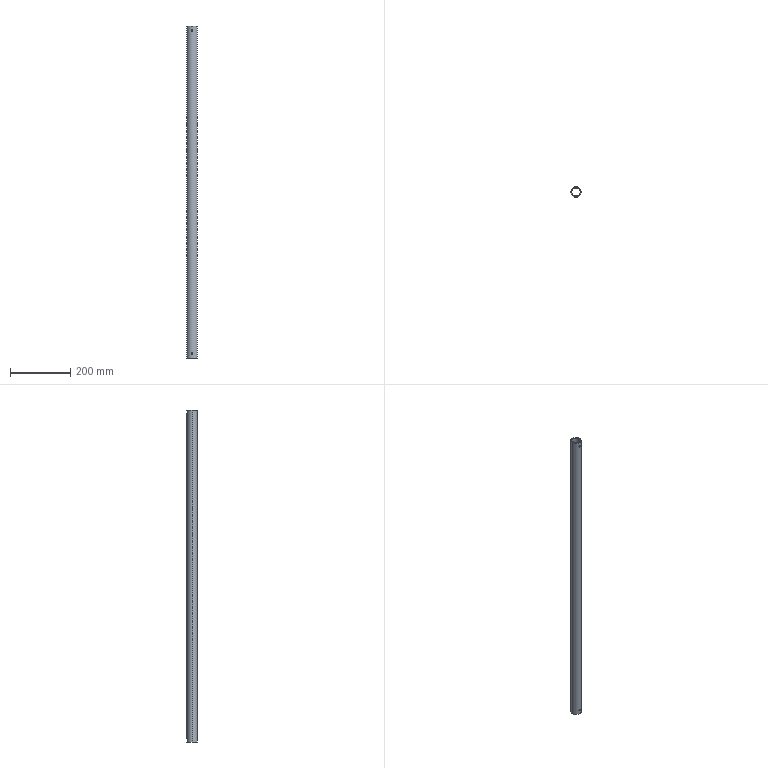Part | SolidWorks | features Extrusion 1, ICE 1 | 1 solid | 14 faces | box 33.7 x 33.7 x 1100 mm | volume 308338 mm3 | cylinder 12 | plane 2 | commonest cylinder face diameters 6 x8 27.9 x2 33.7 x2
STEP:
#1=CARTESIAN_POINT('',(0.,-16.85,12.));
#2=VERTEX_POINT('',#1);
#3=CARTESIAN_POINT('',(0.,-16.85,18.));
#4=VERTEX_POINT('',#3);
#5=CARTESIAN_POINT('',(0.,-16.85,12.));
#6=CARTESIAN_POINT('',(-0.196,-16.85,12.));
#7=CARTESIAN_POINT('',(-0.391,-16.847,12.019));
#8=CARTESIAN_POINT('',(-0.7792,-16.833,12.096));
#9=CARTESIAN_POINT('',(-0.9679,-16.823,12.154));
#10=CARTESIAN_POINT('',(-1.329,-16.798,12.303));
#11=CARTESIAN_POINT('',(-1.504,-16.784,12.397));
#12=CARTESIAN_POINT('',(-1.831,-16.751,12.615));
#13=CARTESIAN_POINT('',(-1.982,-16.734,12.739));
#14=CARTESIAN_POINT('',(-2.258,-16.699,13.016));
#15=CARTESIAN_POINT('',(-2.385,-16.681,13.17));
#16=CARTESIAN_POINT('',(-2.602,-16.648,13.495));
#17=CARTESIAN_POINT('',(-2.695,-16.633,13.667));
#18=CARTESIAN_POINT('',(-2.846,-16.608,14.03));
#19=CARTESIAN_POINT('',(-2.904,-16.598,14.22));
#20=CARTESIAN_POINT('',(-2.98,-16.584,14.604));
#21=CARTESIAN_POINT('',(-3.,-16.581,14.8));
#22=CARTESIAN_POINT('',(-3.,-16.581,15.196));
#23=CARTESIAN_POINT('',(-2.981,-16.584,15.392));
#24=CARTESIAN_POINT('',(-2.905,-16.598,15.776));
#25=CARTESIAN_POINT('',(-2.847,-16.608,15.967));
#26=CARTESIAN_POINT('',(-2.696,-16.633,16.329));
#27=CARTESIAN_POINT('',(-2.604,-16.648,16.502));
#28=CARTESIAN_POINT('',(-2.387,-16.68,16.828));
#29=CARTESIAN_POINT('',(-2.261,-16.698,16.982));
#30=CARTESIAN_POINT('',(-1.847,-16.751,17.396));
#31=CARTESIAN_POINT('',(-1.513,-16.786,17.62));
#32=CARTESIAN_POINT('',(-0.972,-16.823,17.845));
#33=CARTESIAN_POINT('',(-0.7821,-16.833,17.903));
#34=CARTESIAN_POINT('',(-0.3947,-16.846,17.98));
#35=CARTESIAN_POINT('',(-0.1986,-16.85,18.));
#36=CARTESIAN_POINT('',(0.,-16.85,18.));
#37=B_SPLINE_CURVE_WITH_KNOTS('',3,(#5,#6,#7,#8,#9,#10,#11,#12,#13,#14,#15,#16,#17,#18,#19,#20,#21,#22,#23,#24,#25,#26,#27,#28,#29,#30,#31,#32,#33,#34,#35,#36),.UNSPECIFIED.,.F.,.F.,(4,2,2,2,2,2,2,2,2,2,2,2,2,2,2,4),(0.009398,0.009985,0.01057,0.01116,0.01175,0.01233,0.01292,0.01351,0.0141,0.01468,0.01527,0.01586,0.01644,0.01762,0.01821,0.01879),.UNSPECIFIED.);
#38=EDGE_CURVE('',#2,#4,#37,.T.);
#39=ORIENTED_EDGE('',*,*,#38,.F.);
#40=CARTESIAN_POINT('',(0.,-13.95,12.));
#41=VERTEX_POINT('',#40);
#42=CARTESIAN_POINT('',(0.,-16.85,12.));
#43=DIRECTION('',(0.,1.,0.));
#44=VECTOR('',#43,1000.);
#45=LINE('',#42,#44);
#46=EDGE_CURVE('',#2,#41,#45,.T.);
#47=ORIENTED_EDGE('',*,*,#46,.T.);
#48=CARTESIAN_POINT('',(0.,-13.95,18.));
#49=VERTEX_POINT('',#48);
#50=CARTESIAN_POINT('',(0.,-13.95,12.));
#51=CARTESIAN_POINT('',(-0.3921,-13.95,12.));
#52=CARTESIAN_POINT('',(-0.788,-13.932,12.079));
#53=CARTESIAN_POINT('',(-1.33,-13.888,12.304));
#54=CARTESIAN_POINT('',(-1.505,-13.87,12.397));
#55=CARTESIAN_POINT('',(-1.831,-13.83,12.616));
#56=CARTESIAN_POINT('',(-1.982,-13.809,12.739));
#57=CARTESIAN_POINT('',(-2.259,-13.767,13.016));
#58=CARTESIAN_POINT('',(-2.385,-13.745,13.17));
#59=CARTESIAN_POINT('',(-2.602,-13.706,13.494));
#60=CARTESIAN_POINT('',(-2.694,-13.688,13.666));
#61=CARTESIAN_POINT('',(-2.922,-13.642,14.212));
#62=CARTESIAN_POINT('',(-3.,-13.624,14.603));
#63=CARTESIAN_POINT('',(-3.,-13.624,15.197));
#64=CARTESIAN_POINT('',(-2.981,-13.628,15.392));
#65=CARTESIAN_POINT('',(-2.904,-13.644,15.776));
#66=CARTESIAN_POINT('',(-2.846,-13.657,15.968));
#67=CARTESIAN_POINT('',(-2.696,-13.687,16.33));
#68=CARTESIAN_POINT('',(-2.604,-13.705,16.502));
#69=CARTESIAN_POINT('',(-2.386,-13.745,16.829));
#70=CARTESIAN_POINT('',(-2.26,-13.766,16.982));
#71=CARTESIAN_POINT('',(-1.847,-13.83,17.396));
#72=CARTESIAN_POINT('',(-1.514,-13.872,17.619));
#73=CARTESIAN_POINT('',(-0.9725,-13.917,17.845));
#74=CARTESIAN_POINT('',(-0.7819,-13.929,17.903));
#75=CARTESIAN_POINT('',(-0.3949,-13.946,17.98));
#76=CARTESIAN_POINT('',(-0.1988,-13.95,18.));
#77=CARTESIAN_POINT('',(0.,-13.95,18.));
#78=B_SPLINE_CURVE_WITH_KNOTS('',3,(#50,#51,#52,#53,#54,#55,#56,#57,#58,#59,#60,#61,#62,#63,#64,#65,#66,#67,#68,#69,#70,#71,#72,#73,#74,#75,#76,#77),.UNSPECIFIED.,.F.,.F.,(4,2,2,2,2,2,2,2,2,2,2,2,2,4),(0.009407,0.01058,0.01117,0.01176,0.01235,0.01293,0.01411,0.0147,0.01528,0.01587,0.01646,0.01764,0.01822,0.01881),.UNSPECIFIED.);
#79=EDGE_CURVE('',#41,#49,#78,.T.);
#80=ORIENTED_EDGE('',*,*,#79,.T.);
#81=CARTESIAN_POINT('',(0.,-16.85,18.));
#82=DIRECTION('',(0.,1.,0.));
#83=VECTOR('',#82,1000.);
#84=LINE('',#81,#83);
#85=EDGE_CURVE('',#4,#49,#84,.T.);
#86=ORIENTED_EDGE('',*,*,#85,.F.);
#87=EDGE_LOOP('',(#39,#47,#80,#86));
#88=FACE_OUTER_BOUND('',#87,.T.);
#89=CARTESIAN_POINT('',(0.,-16.85,15.));
#90=DIRECTION('',(0.,1.,0.));
#91=DIRECTION('',(0.,0.,1.));
#92=AXIS2_PLACEMENT_3D('',#89,#90,#91);
#93=CYLINDRICAL_SURFACE('',#92,3.);
#94=ADVANCED_FACE('',(#88),#93,.F.);
#95=CARTESIAN_POINT('',(0.,13.95,18.));
#96=VERTEX_POINT('',#95);
#97=CARTESIAN_POINT('',(0.,13.95,12.));
#98=VERTEX_POINT('',#97);
#99=CARTESIAN_POINT('',(0.,13.95,18.));
#100=CARTESIAN_POINT('',(-0.1988,13.95,18.));
#101=CARTESIAN_POINT('',(-0.3942,13.946,17.98));
#102=CARTESIAN_POINT('',(-0.7785,13.93,17.904));
#103=CARTESIAN_POINT('',(-0.9694,13.917,17.846));
#104=CARTESIAN_POINT('',(-1.332,13.887,17.695));
#105=CARTESIAN_POINT('',(-1.505,13.87,17.603));
#106=CARTESIAN_POINT('',(-1.83,13.83,17.385));
#107=CARTESIAN_POINT('',(-1.984,13.809,17.259));
#108=CARTESIAN_POINT('',(-2.26,13.766,16.983));
#109=CARTESIAN_POINT('',(-2.384,13.745,16.832));
#110=CARTESIAN_POINT('',(-2.603,13.705,16.504));
#111=CARTESIAN_POINT('',(-2.696,13.687,16.331));
#112=CARTESIAN_POINT('',(-2.846,13.657,15.97));
#113=CARTESIAN_POINT('',(-2.904,13.645,15.78));
#114=CARTESIAN_POINT('',(-2.981,13.628,15.393));
#115=CARTESIAN_POINT('',(-3.,13.624,15.198));
#116=CARTESIAN_POINT('',(-3.,13.624,14.805));
#117=CARTESIAN_POINT('',(-2.98,13.628,14.605));
#118=CARTESIAN_POINT('',(-2.904,13.645,14.22));
#119=CARTESIAN_POINT('',(-2.847,13.657,14.033));
#120=CARTESIAN_POINT('',(-2.696,13.687,13.669));
#121=CARTESIAN_POINT('',(-2.602,13.706,13.494));
#122=CARTESIAN_POINT('',(-2.385,13.745,13.17));
#123=CARTESIAN_POINT('',(-2.26,13.766,13.018));
#124=CARTESIAN_POINT('',(-1.982,13.809,12.739));
#125=CARTESIAN_POINT('',(-1.831,13.83,12.615));
#126=CARTESIAN_POINT('',(-1.506,13.869,12.398));
#127=CARTESIAN_POINT('',(-1.331,13.888,12.304));
#128=CARTESIAN_POINT('',(-0.9682,13.918,12.154));
#129=CARTESIAN_POINT('',(-0.7811,13.929,12.097));
#130=CARTESIAN_POINT('',(-0.3953,13.946,12.02));
#131=CARTESIAN_POINT('',(-0.1961,13.95,12.));
#132=CARTESIAN_POINT('',(0.,13.95,12.));
#133=B_SPLINE_CURVE_WITH_KNOTS('',3,(#99,#100,#101,#102,#103,#104,#105,#106,#107,#108,#109,#110,#111,#112,#113,#114,#115,#116,#117,#118,#119,#120,#121,#122,#123,#124,#125,#126,#127,#128,#129,#130,#131,#132),.UNSPECIFIED.,.F.,.F.,(4,2,2,2,2,2,2,2,2,2,2,2,2,2,2,2,4),(0.,0.0005879,0.001176,0.001764,0.002352,0.00294,0.003528,0.004116,0.004703,0.005291,0.005879,0.006467,0.007055,0.007643,0.008231,0.008819,0.009407),.UNSPECIFIED.);
#134=EDGE_CURVE('',#96,#98,#133,.T.);
#135=ORIENTED_EDGE('',*,*,#134,.T.);
#136=CARTESIAN_POINT('',(0.,16.85,12.));
#137=VERTEX_POINT('',#136);
#138=CARTESIAN_POINT('',(0.,-16.85,12.));
#139=DIRECTION('',(0.,1.,0.));
#140=VECTOR('',#139,1000.);
#141=LINE('',#138,#140);
#142=EDGE_CURVE('',#98,#137,#141,.T.);
#143=ORIENTED_EDGE('',*,*,#142,.T.);
#144=CARTESIAN_POINT('',(0.,16.85,18.));
#145=VERTEX_POINT('',#144);
#146=CARTESIAN_POINT('',(0.,16.85,18.));
#147=CARTESIAN_POINT('',(-0.1986,16.85,18.));
#148=CARTESIAN_POINT('',(-0.3939,16.846,17.98));
#149=CARTESIAN_POINT('',(-0.7779,16.833,17.904));
#150=CARTESIAN_POINT('',(-0.9687,16.823,17.846));
#151=CARTESIAN_POINT('',(-1.332,16.798,17.695));
#152=CARTESIAN_POINT('',(-1.504,16.784,17.603));
#153=CARTESIAN_POINT('',(-1.83,16.751,17.385));
#154=CARTESIAN_POINT('',(-1.984,16.733,17.259));
#155=CARTESIAN_POINT('',(-2.26,16.698,16.983));
#156=CARTESIAN_POINT('',(-2.384,16.681,16.832));
#157=CARTESIAN_POINT('',(-2.603,16.648,16.504));
#158=CARTESIAN_POINT('',(-2.696,16.633,16.33));
#159=CARTESIAN_POINT('',(-2.846,16.608,15.969));
#160=CARTESIAN_POINT('',(-2.904,16.598,15.78));
#161=CARTESIAN_POINT('',(-2.981,16.584,15.392));
#162=CARTESIAN_POINT('',(-3.,16.581,15.197));
#163=CARTESIAN_POINT('',(-3.,16.581,14.805));
#164=CARTESIAN_POINT('',(-2.98,16.584,14.606));
#165=CARTESIAN_POINT('',(-2.904,16.598,14.221));
#166=CARTESIAN_POINT('',(-2.847,16.608,14.034));
#167=CARTESIAN_POINT('',(-2.696,16.633,13.67));
#168=CARTESIAN_POINT('',(-2.602,16.648,13.495));
#169=CARTESIAN_POINT('',(-2.385,16.681,13.17));
#170=CARTESIAN_POINT('',(-2.261,16.698,13.018));
#171=CARTESIAN_POINT('',(-1.982,16.734,12.739));
#172=CARTESIAN_POINT('',(-1.831,16.751,12.615));
#173=CARTESIAN_POINT('',(-1.506,16.783,12.398));
#174=CARTESIAN_POINT('',(-1.33,16.798,12.304));
#175=CARTESIAN_POINT('',(-0.9675,16.823,12.154));
#176=CARTESIAN_POINT('',(-0.7805,16.833,12.097));
#177=CARTESIAN_POINT('',(-0.3951,16.846,12.02));
#178=CARTESIAN_POINT('',(-0.196,16.85,12.));
#179=CARTESIAN_POINT('',(0.,16.85,12.));
#180=B_SPLINE_CURVE_WITH_KNOTS('',3,(#146,#147,#148,#149,#150,#151,#152,#153,#154,#155,#156,#157,#158,#159,#160,#161,#162,#163,#164,#165,#166,#167,#168,#169,#170,#171,#172,#173,#174,#175,#176,#177,#178,#179),.UNSPECIFIED.,.F.,.F.,(4,2,2,2,2,2,2,2,2,2,2,2,2,2,2,2,4),(0.,0.0005874,0.001175,0.001762,0.00235,0.002937,0.003524,0.004112,0.004699,0.005286,0.005874,0.006461,0.007049,0.007636,0.008223,0.008811,0.009398),.UNSPECIFIED.);
#181=EDGE_CURVE('',#145,#137,#180,.T.);
#182=ORIENTED_EDGE('',*,*,#181,.F.);
#183=CARTESIAN_POINT('',(0.,-16.85,18.));
#184=DIRECTION('',(0.,1.,0.));
#185=VECTOR('',#184,1000.);
#186=LINE('',#183,#185);
#187=EDGE_CURVE('',#96,#145,#186,.T.);
#188=ORIENTED_EDGE('',*,*,#187,.F.);
#189=EDGE_LOOP('',(#135,#143,#182,#188));
#190=FACE_OUTER_BOUND('',#189,.T.);
#191=CARTESIAN_POINT('',(0.,-16.85,15.));
#192=DIRECTION('',(0.,1.,0.));
#193=DIRECTION('',(0.,0.,1.));
#194=AXIS2_PLACEMENT_3D('',#191,#192,#193);
#195=CYLINDRICAL_SURFACE('',#194,3.);
#196=ADVANCED_FACE('',(#190),#195,.F.);
#197=CARTESIAN_POINT('',(0.,-16.85,1082.));
#198=VERTEX_POINT('',#197);
#199=CARTESIAN_POINT('',(0.,-16.85,1088.));
#200=VERTEX_POINT('',#199);
#201=CARTESIAN_POINT('',(0.,-16.85,1082.));
#202=CARTESIAN_POINT('',(-0.196,-16.85,1082.));
#203=CARTESIAN_POINT('',(-0.391,-16.847,1082.019));
#204=CARTESIAN_POINT('',(-0.7792,-16.833,1082.096));
#205=CARTESIAN_POINT('',(-0.9679,-16.823,1082.154));
#206=CARTESIAN_POINT('',(-1.329,-16.798,1082.303));
#207=CARTESIAN_POINT('',(-1.504,-16.784,1082.397));
#208=CARTESIAN_POINT('',(-1.831,-16.751,1082.615));
#209=CARTESIAN_POINT('',(-1.982,-16.734,1082.739));
#210=CARTESIAN_POINT('',(-2.258,-16.699,1083.016));
#211=CARTESIAN_POINT('',(-2.385,-16.681,1083.17));
#212=CARTESIAN_POINT('',(-2.602,-16.648,1083.495));
#213=CARTESIAN_POINT('',(-2.695,-16.633,1083.667));
#214=CARTESIAN_POINT('',(-2.846,-16.608,1084.03));
#215=CARTESIAN_POINT('',(-2.904,-16.598,1084.22));
#216=CARTESIAN_POINT('',(-2.98,-16.584,1084.604));
#217=CARTESIAN_POINT('',(-3.,-16.581,1084.8));
#218=CARTESIAN_POINT('',(-3.,-16.581,1085.196));
#219=CARTESIAN_POINT('',(-2.981,-16.584,1085.392));
#220=CARTESIAN_POINT('',(-2.905,-16.598,1085.776));
#221=CARTESIAN_POINT('',(-2.847,-16.608,1085.967));
#222=CARTESIAN_POINT('',(-2.696,-16.633,1086.329));
#223=CARTESIAN_POINT('',(-2.604,-16.648,1086.502));
#224=CARTESIAN_POINT('',(-2.387,-16.68,1086.828));
#225=CARTESIAN_POINT('',(-2.261,-16.698,1086.982));
#226=CARTESIAN_POINT('',(-1.847,-16.751,1087.396));
#227=CARTESIAN_POINT('',(-1.513,-16.786,1087.62));
#228=CARTESIAN_POINT('',(-0.972,-16.823,1087.845));
#229=CARTESIAN_POINT('',(-0.7821,-16.833,1087.903));
#230=CARTESIAN_POINT('',(-0.3947,-16.846,1087.98));
#231=CARTESIAN_POINT('',(-0.1986,-16.85,1088.));
#232=CARTESIAN_POINT('',(0.,-16.85,1088.));
#233=B_SPLINE_CURVE_WITH_KNOTS('',3,(#201,#202,#203,#204,#205,#206,#207,#208,#209,#210,#211,#212,#213,#214,#215,#216,#217,#218,#219,#220,#221,#222,#223,#224,#225,#226,#227,#228,#229,#230,#231,#232),.UNSPECIFIED.,.F.,.F.,(4,2,2,2,2,2,2,2,2,2,2,2,2,2,2,4),(0.009398,0.009985,0.01057,0.01116,0.01175,0.01233,0.01292,0.01351,0.0141,0.01468,0.01527,0.01586,0.01644,0.01762,0.01821,0.01879),.UNSPECIFIED.);
#234=EDGE_CURVE('',#198,#200,#233,.T.);
#235=ORIENTED_EDGE('',*,*,#234,.F.);
#236=CARTESIAN_POINT('',(0.,-13.95,1082.));
#237=VERTEX_POINT('',#236);
#238=CARTESIAN_POINT('',(0.,-16.85,1082.));
#239=DIRECTION('',(0.,1.,0.));
#240=VECTOR('',#239,1000.);
#241=LINE('',#238,#240);
#242=EDGE_CURVE('',#198,#237,#241,.T.);
#243=ORIENTED_EDGE('',*,*,#242,.T.);
#244=CARTESIAN_POINT('',(0.,-13.95,1088.));
#245=VERTEX_POINT('',#244);
#246=CARTESIAN_POINT('',(0.,-13.95,1082.));
#247=CARTESIAN_POINT('',(-0.3921,-13.95,1082.));
#248=CARTESIAN_POINT('',(-0.788,-13.932,1082.079));
#249=CARTESIAN_POINT('',(-1.33,-13.888,1082.304));
#250=CARTESIAN_POINT('',(-1.505,-13.87,1082.397));
#251=CARTESIAN_POINT('',(-1.831,-13.83,1082.616));
#252=CARTESIAN_POINT('',(-1.982,-13.809,1082.739));
#253=CARTESIAN_POINT('',(-2.259,-13.767,1083.016));
#254=CARTESIAN_POINT('',(-2.385,-13.745,1083.17));
#255=CARTESIAN_POINT('',(-2.602,-13.706,1083.494));
#256=CARTESIAN_POINT('',(-2.694,-13.688,1083.666));
#257=CARTESIAN_POINT('',(-2.922,-13.642,1084.212));
#258=CARTESIAN_POINT('',(-3.,-13.624,1084.603));
#259=CARTESIAN_POINT('',(-3.,-13.624,1085.197));
#260=CARTESIAN_POINT('',(-2.981,-13.628,1085.392));
#261=CARTESIAN_POINT('',(-2.904,-13.644,1085.776));
#262=CARTESIAN_POINT('',(-2.846,-13.657,1085.968));
#263=CARTESIAN_POINT('',(-2.696,-13.687,1086.33));
#264=CARTESIAN_POINT('',(-2.604,-13.705,1086.502));
#265=CARTESIAN_POINT('',(-2.386,-13.745,1086.829));
#266=CARTESIAN_POINT('',(-2.26,-13.766,1086.982));
#267=CARTESIAN_POINT('',(-1.847,-13.83,1087.396));
#268=CARTESIAN_POINT('',(-1.514,-13.872,1087.619));
#269=CARTESIAN_POINT('',(-0.9725,-13.917,1087.845));
#270=CARTESIAN_POINT('',(-0.7819,-13.929,1087.903));
#271=CARTESIAN_POINT('',(-0.3949,-13.946,1087.98));
#272=CARTESIAN_POINT('',(-0.1988,-13.95,1088.));
#273=CARTESIAN_POINT('',(0.,-13.95,1088.));
#274=B_SPLINE_CURVE_WITH_KNOTS('',3,(#246,#247,#248,#249,#250,#251,#252,#253,#254,#255,#256,#257,#258,#259,#260,#261,#262,#263,#264,#265,#266,#267,#268,#269,#270,#271,#272,#273),.UNSPECIFIED.,.F.,.F.,(4,2,2,2,2,2,2,2,2,2,2,2,2,4),(0.009407,0.01058,0.01117,0.01176,0.01235,0.01293,0.01411,0.0147,0.01528,0.01587,0.01646,0.01764,0.01822,0.01881),.UNSPECIFIED.);
#275=EDGE_CURVE('',#237,#245,#274,.T.);
#276=ORIENTED_EDGE('',*,*,#275,.T.);
#277=CARTESIAN_POINT('',(0.,-16.85,1088.));
#278=DIRECTION('',(0.,1.,0.));
#279=VECTOR('',#278,1000.);
#280=LINE('',#277,#279);
#281=EDGE_CURVE('',#200,#245,#280,.T.);
#282=ORIENTED_EDGE('',*,*,#281,.F.);
#283=EDGE_LOOP('',(#235,#243,#276,#282));
#284=FACE_OUTER_BOUND('',#283,.T.);
#285=CARTESIAN_POINT('',(0.,-16.85,1085.));
#286=DIRECTION('',(0.,1.,0.));
#287=DIRECTION('',(0.,0.,1.));
#288=AXIS2_PLACEMENT_3D('',#285,#286,#287);
#289=CYLINDRICAL_SURFACE('',#288,3.);
#290=ADVANCED_FACE('',(#284),#289,.F.);
#291=CARTESIAN_POINT('',(0.,13.95,1088.));
#292=VERTEX_POINT('',#291);
#293=CARTESIAN_POINT('',(0.,13.95,1082.));
#294=VERTEX_POINT('',#293);
#295=CARTESIAN_POINT('',(0.,13.95,1088.));
#296=CARTESIAN_POINT('',(-0.1988,13.95,1088.));
#297=CARTESIAN_POINT('',(-0.3942,13.946,1087.98));
#298=CARTESIAN_POINT('',(-0.7785,13.93,1087.904));
#299=CARTESIAN_POINT('',(-0.9694,13.917,1087.846));
#300=CARTESIAN_POINT('',(-1.332,13.887,1087.695));
#301=CARTESIAN_POINT('',(-1.505,13.87,1087.603));
#302=CARTESIAN_POINT('',(-1.83,13.83,1087.385));
#303=CARTESIAN_POINT('',(-1.984,13.809,1087.259));
#304=CARTESIAN_POINT('',(-2.26,13.766,1086.983));
#305=CARTESIAN_POINT('',(-2.384,13.745,1086.832));
#306=CARTESIAN_POINT('',(-2.603,13.705,1086.504));
#307=CARTESIAN_POINT('',(-2.696,13.687,1086.331));
#308=CARTESIAN_POINT('',(-2.846,13.657,1085.97));
#309=CARTESIAN_POINT('',(-2.904,13.645,1085.78));
#310=CARTESIAN_POINT('',(-2.981,13.628,1085.393));
#311=CARTESIAN_POINT('',(-3.,13.624,1085.198));
#312=CARTESIAN_POINT('',(-3.,13.624,1084.805));
#313=CARTESIAN_POINT('',(-2.98,13.628,1084.605));
#314=CARTESIAN_POINT('',(-2.904,13.645,1084.22));
#315=CARTESIAN_POINT('',(-2.847,13.657,1084.033));
#316=CARTESIAN_POINT('',(-2.696,13.687,1083.669));
#317=CARTESIAN_POINT('',(-2.602,13.706,1083.494));
#318=CARTESIAN_POINT('',(-2.385,13.745,1083.17));
#319=CARTESIAN_POINT('',(-2.26,13.766,1083.018));
#320=CARTESIAN_POINT('',(-1.982,13.809,1082.739));
#321=CARTESIAN_POINT('',(-1.831,13.83,1082.615));
#322=CARTESIAN_POINT('',(-1.506,13.869,1082.398));
#323=CARTESIAN_POINT('',(-1.331,13.888,1082.304));
#324=CARTESIAN_POINT('',(-0.9682,13.918,1082.154));
#325=CARTESIAN_POINT('',(-0.7811,13.929,1082.097));
#326=CARTESIAN_POINT('',(-0.3953,13.946,1082.02));
#327=CARTESIAN_POINT('',(-0.1961,13.95,1082.));
#328=CARTESIAN_POINT('',(0.,13.95,1082.));
#329=B_SPLINE_CURVE_WITH_KNOTS('',3,(#295,#296,#297,#298,#299,#300,#301,#302,#303,#304,#305,#306,#307,#308,#309,#310,#311,#312,#313,#314,#315,#316,#317,#318,#319,#320,#321,#322,#323,#324,#325,#326,#327,#328),.UNSPECIFIED.,.F.,.F.,(4,2,2,2,2,2,2,2,2,2,2,2,2,2,2,2,4),(0.,0.0005879,0.001176,0.001764,0.002352,0.00294,0.003528,0.004116,0.004703,0.005291,0.005879,0.006467,0.007055,0.007643,0.008231,0.008819,0.009407),.UNSPECIFIED.);
#330=EDGE_CURVE('',#292,#294,#329,.T.);
#331=ORIENTED_EDGE('',*,*,#330,.T.);
#332=CARTESIAN_POINT('',(0.,16.85,1082.));
#333=VERTEX_POINT('',#332);
#334=CARTESIAN_POINT('',(0.,-16.85,1082.));
#335=DIRECTION('',(0.,1.,0.));
#336=VECTOR('',#335,1000.);
#337=LINE('',#334,#336);
#338=EDGE_CURVE('',#294,#333,#337,.T.);
#339=ORIENTED_EDGE('',*,*,#338,.T.);
#340=CARTESIAN_POINT('',(0.,16.85,1088.));
#341=VERTEX_POINT('',#340);
#342=CARTESIAN_POINT('',(0.,16.85,1088.));
#343=CARTESIAN_POINT('',(-0.1986,16.85,1088.));
#344=CARTESIAN_POINT('',(-0.3939,16.846,1087.98));
#345=CARTESIAN_POINT('',(-0.7779,16.833,1087.904));
#346=CARTESIAN_POINT('',(-0.9687,16.823,1087.846));
#347=CARTESIAN_POINT('',(-1.332,16.798,1087.695));
#348=CARTESIAN_POINT('',(-1.504,16.784,1087.603));
#349=CARTESIAN_POINT('',(-1.83,16.751,1087.385));
#350=CARTESIAN_POINT('',(-1.984,16.733,1087.259));
#351=CARTESIAN_POINT('',(-2.26,16.698,1086.983));
#352=CARTESIAN_POINT('',(-2.384,16.681,1086.832));
#353=CARTESIAN_POINT('',(-2.603,16.648,1086.504));
#354=CARTESIAN_POINT('',(-2.696,16.633,1086.33));
#355=CARTESIAN_POINT('',(-2.846,16.608,1085.969));
#356=CARTESIAN_POINT('',(-2.904,16.598,1085.78));
#357=CARTESIAN_POINT('',(-2.981,16.584,1085.392));
#358=CARTESIAN_POINT('',(-3.,16.581,1085.197));
#359=CARTESIAN_POINT('',(-3.,16.581,1084.805));
#360=CARTESIAN_POINT('',(-2.98,16.584,1084.606));
#361=CARTESIAN_POINT('',(-2.904,16.598,1084.221));
#362=CARTESIAN_POINT('',(-2.847,16.608,1084.034));
#363=CARTESIAN_POINT('',(-2.696,16.633,1083.67));
#364=CARTESIAN_POINT('',(-2.602,16.648,1083.495));
#365=CARTESIAN_POINT('',(-2.385,16.681,1083.17));
#366=CARTESIAN_POINT('',(-2.261,16.698,1083.018));
#367=CARTESIAN_POINT('',(-1.982,16.734,1082.739));
#368=CARTESIAN_POINT('',(-1.831,16.751,1082.615));
#369=CARTESIAN_POINT('',(-1.506,16.783,1082.398));
#370=CARTESIAN_POINT('',(-1.33,16.798,1082.304));
#371=CARTESIAN_POINT('',(-0.9675,16.823,1082.154));
#372=CARTESIAN_POINT('',(-0.7805,16.833,1082.097));
#373=CARTESIAN_POINT('',(-0.3951,16.846,1082.02));
#374=CARTESIAN_POINT('',(-0.196,16.85,1082.));
#375=CARTESIAN_POINT('',(0.,16.85,1082.));
#376=B_SPLINE_CURVE_WITH_KNOTS('',3,(#342,#343,#344,#345,#346,#347,#348,#349,#350,#351,#352,#353,#354,#355,#356,#357,#358,#359,#360,#361,#362,#363,#364,#365,#366,#367,#368,#369,#370,#371,#372,#373,#374,#375),.UNSPECIFIED.,.F.,.F.,(4,2,2,2,2,2,2,2,2,2,2,2,2,2,2,2,4),(0.,0.0005874,0.001175,0.001762,0.00235,0.002937,0.003524,0.004112,0.004699,0.005286,0.005874,0.006461,0.007049,0.007636,0.008223,0.008811,0.009398),.UNSPECIFIED.);
#377=EDGE_CURVE('',#341,#333,#376,.T.);
#378=ORIENTED_EDGE('',*,*,#377,.F.);
#379=CARTESIAN_POINT('',(0.,-16.85,1088.));
#380=DIRECTION('',(0.,1.,0.));
#381=VECTOR('',#380,1000.);
#382=LINE('',#379,#381);
#383=EDGE_CURVE('',#292,#341,#382,.T.);
#384=ORIENTED_EDGE('',*,*,#383,.F.);
#385=EDGE_LOOP('',(#331,#339,#378,#384));
#386=FACE_OUTER_BOUND('',#385,.T.);
#387=CARTESIAN_POINT('',(0.,-16.85,1085.));
#388=DIRECTION('',(0.,1.,0.));
#389=DIRECTION('',(0.,0.,1.));
#390=AXIS2_PLACEMENT_3D('',#387,#388,#389);
#391=CYLINDRICAL_SURFACE('',#390,3.);
#392=ADVANCED_FACE('',(#386),#391,.F.);
#393=CARTESIAN_POINT('',(0.,-13.95,1088.));
#394=CARTESIAN_POINT('',(0.1988,-13.95,1088.));
#395=CARTESIAN_POINT('',(0.3942,-13.946,1087.98));
#396=CARTESIAN_POINT('',(0.7785,-13.93,1087.904));
#397=CARTESIAN_POINT('',(0.9694,-13.917,1087.846));
#398=CARTESIAN_POINT('',(1.332,-13.887,1087.695));
#399=CARTESIAN_POINT('',(1.505,-13.87,1087.603));
#400=CARTESIAN_POINT('',(1.83,-13.83,1087.385));
#401=CARTESIAN_POINT('',(1.984,-13.809,1087.259));
#402=CARTESIAN_POINT('',(2.26,-13.766,1086.983));
#403=CARTESIAN_POINT('',(2.384,-13.745,1086.832));
#404=CARTESIAN_POINT('',(2.603,-13.705,1086.504));
#405=CARTESIAN_POINT('',(2.696,-13.687,1086.331));
#406=CARTESIAN_POINT('',(2.846,-13.657,1085.97));
#407=CARTESIAN_POINT('',(2.904,-13.645,1085.78));
#408=CARTESIAN_POINT('',(2.981,-13.628,1085.393));
#409=CARTESIAN_POINT('',(3.,-13.624,1085.198));
#410=CARTESIAN_POINT('',(3.,-13.624,1084.805));
#411=CARTESIAN_POINT('',(2.98,-13.628,1084.605));
#412=CARTESIAN_POINT('',(2.904,-13.645,1084.22));
#413=CARTESIAN_POINT('',(2.847,-13.657,1084.033));
#414=CARTESIAN_POINT('',(2.696,-13.687,1083.669));
#415=CARTESIAN_POINT('',(2.602,-13.706,1083.494));
#416=CARTESIAN_POINT('',(2.385,-13.745,1083.17));
#417=CARTESIAN_POINT('',(2.26,-13.766,1083.018));
#418=CARTESIAN_POINT('',(1.982,-13.809,1082.739));
#419=CARTESIAN_POINT('',(1.831,-13.83,1082.615));
#420=CARTESIAN_POINT('',(1.506,-13.869,1082.398));
#421=CARTESIAN_POINT('',(1.331,-13.888,1082.304));
#422=CARTESIAN_POINT('',(0.9682,-13.918,1082.154));
#423=CARTESIAN_POINT('',(0.7811,-13.929,1082.097));
#424=CARTESIAN_POINT('',(0.3953,-13.946,1082.02));
#425=CARTESIAN_POINT('',(0.1961,-13.95,1082.));
#426=CARTESIAN_POINT('',(0.,-13.95,1082.));
#427=B_SPLINE_CURVE_WITH_KNOTS('',3,(#393,#394,#395,#396,#397,#398,#399,#400,#401,#402,#403,#404,#405,#406,#407,#408,#409,#410,#411,#412,#413,#414,#415,#416,#417,#418,#419,#420,#421,#422,#423,#424,#425,#426),.UNSPECIFIED.,.F.,.F.,(4,2,2,2,2,2,2,2,2,2,2,2,2,2,2,2,4),(0.,0.0005879,0.001176,0.001764,0.002352,0.00294,0.003528,0.004116,0.004703,0.005291,0.005879,0.006467,0.007055,0.007643,0.008231,0.008819,0.009407),.UNSPECIFIED.);
#428=EDGE_CURVE('',#245,#237,#427,.T.);
#429=ORIENTED_EDGE('',*,*,#428,.F.);
#430=ORIENTED_EDGE('',*,*,#275,.F.);
#431=EDGE_LOOP('',(#429,#430));
#432=FACE_BOUND('',#431,.T.);
#433=CARTESIAN_POINT('',(0.,-13.95,18.));
#434=CARTESIAN_POINT('',(0.1988,-13.95,18.));
#435=CARTESIAN_POINT('',(0.3942,-13.946,17.98));
#436=CARTESIAN_POINT('',(0.7785,-13.93,17.904));
#437=CARTESIAN_POINT('',(0.9694,-13.917,17.846));
#438=CARTESIAN_POINT('',(1.332,-13.887,17.695));
#439=CARTESIAN_POINT('',(1.505,-13.87,17.603));
#440=CARTESIAN_POINT('',(1.83,-13.83,17.385));
#441=CARTESIAN_POINT('',(1.984,-13.809,17.259));
#442=CARTESIAN_POINT('',(2.26,-13.766,16.983));
#443=CARTESIAN_POINT('',(2.384,-13.745,16.832));
#444=CARTESIAN_POINT('',(2.603,-13.705,16.504));
#445=CARTESIAN_POINT('',(2.696,-13.687,16.331));
#446=CARTESIAN_POINT('',(2.846,-13.657,15.97));
#447=CARTESIAN_POINT('',(2.904,-13.645,15.78));
#448=CARTESIAN_POINT('',(2.981,-13.628,15.393));
#449=CARTESIAN_POINT('',(3.,-13.624,15.198));
#450=CARTESIAN_POINT('',(3.,-13.624,14.805));
#451=CARTESIAN_POINT('',(2.98,-13.628,14.605));
#452=CARTESIAN_POINT('',(2.904,-13.645,14.22));
#453=CARTESIAN_POINT('',(2.847,-13.657,14.033));
#454=CARTESIAN_POINT('',(2.696,-13.687,13.669));
#455=CARTESIAN_POINT('',(2.602,-13.706,13.494));
#456=CARTESIAN_POINT('',(2.385,-13.745,13.17));
#457=CARTESIAN_POINT('',(2.26,-13.766,13.018));
#458=CARTESIAN_POINT('',(1.982,-13.809,12.739));
#459=CARTESIAN_POINT('',(1.831,-13.83,12.615));
#460=CARTESIAN_POINT('',(1.506,-13.869,12.398));
#461=CARTESIAN_POINT('',(1.331,-13.888,12.304));
#462=CARTESIAN_POINT('',(0.9682,-13.918,12.154));
#463=CARTESIAN_POINT('',(0.7811,-13.929,12.097));
#464=CARTESIAN_POINT('',(0.3953,-13.946,12.02));
#465=CARTESIAN_POINT('',(0.1961,-13.95,12.));
#466=CARTESIAN_POINT('',(0.,-13.95,12.));
#467=B_SPLINE_CURVE_WITH_KNOTS('',3,(#433,#434,#435,#436,#437,#438,#439,#440,#441,#442,#443,#444,#445,#446,#447,#448,#449,#450,#451,#452,#453,#454,#455,#456,#457,#458,#459,#460,#461,#462,#463,#464,#465,#466),.UNSPECIFIED.,.F.,.F.,(4,2,2,2,2,2,2,2,2,2,2,2,2,2,2,2,4),(0.,0.0005879,0.001176,0.001764,0.002352,0.00294,0.003528,0.004116,0.004703,0.005291,0.005879,0.006467,0.007055,0.007643,0.008231,0.008819,0.009407),.UNSPECIFIED.);
#468=EDGE_CURVE('',#49,#41,#467,.T.);
#469=ORIENTED_EDGE('',*,*,#468,.F.);
#470=ORIENTED_EDGE('',*,*,#79,.F.);
#471=EDGE_LOOP('',(#469,#470));
#472=FACE_BOUND('',#471,.T.);
#473=CARTESIAN_POINT('',(-13.95,0.,1100.));
#474=VERTEX_POINT('',#473);
#475=CARTESIAN_POINT('',(13.95,0.,1100.));
#476=VERTEX_POINT('',#475);
#477=CARTESIAN_POINT('',(0.,0.,1100.));
#478=DIRECTION('',(0.,0.,1.));
#479=DIRECTION('',(1.,0.,0.));
#480=AXIS2_PLACEMENT_3D('',#477,#478,#479);
#481=CIRCLE('',#480,13.95);
#482=EDGE_CURVE('',#474,#476,#481,.T.);
#483=ORIENTED_EDGE('',*,*,#482,.T.);
#484=CARTESIAN_POINT('',(13.95,0.,0.));
#485=VERTEX_POINT('',#484);
#486=CARTESIAN_POINT('',(13.95,0.,1100.));
#487=DIRECTION('',(0.,0.,-1.));
#488=VECTOR('',#487,1000.);
#489=LINE('',#486,#488);
#490=EDGE_CURVE('',#476,#485,#489,.T.);
#491=ORIENTED_EDGE('',*,*,#490,.T.);
#492=CARTESIAN_POINT('',(-13.95,0.,0.));
#493=VERTEX_POINT('',#492);
#494=CARTESIAN_POINT('',(0.,0.,0.));
#495=DIRECTION('',(0.,0.,1.));
#496=DIRECTION('',(1.,0.,0.));
#497=AXIS2_PLACEMENT_3D('',#494,#495,#496);
#498=CIRCLE('',#497,13.95);
#499=EDGE_CURVE('',#493,#485,#498,.T.);
#500=ORIENTED_EDGE('',*,*,#499,.F.);
#501=CARTESIAN_POINT('',(-13.95,0.,1100.));
#502=DIRECTION('',(0.,0.,-1.));
#503=VECTOR('',#502,1000.);
#504=LINE('',#501,#503);
#505=EDGE_CURVE('',#474,#493,#504,.T.);
#506=ORIENTED_EDGE('',*,*,#505,.F.);
#507=EDGE_LOOP('',(#483,#491,#500,#506));
#508=FACE_OUTER_BOUND('',#507,.T.);
#509=CARTESIAN_POINT('',(0.,0.,1100.));
#510=DIRECTION('',(0.,0.,-1.));
#511=DIRECTION('',(-1.,0.,0.));
#512=AXIS2_PLACEMENT_3D('',#509,#510,#511);
#513=CYLINDRICAL_SURFACE('',#512,13.95);
#514=ADVANCED_FACE('',(#432,#472,#508),#513,.F.);
#515=ORIENTED_EDGE('',*,*,#377,.T.);
#516=CARTESIAN_POINT('',(0.,16.85,1082.));
#517=CARTESIAN_POINT('',(0.196,16.85,1082.));
#518=CARTESIAN_POINT('',(0.391,16.847,1082.019));
#519=CARTESIAN_POINT('',(0.7792,16.833,1082.096));
#520=CARTESIAN_POINT('',(0.9679,16.823,1082.154));
#521=CARTESIAN_POINT('',(1.329,16.798,1082.303));
#522=CARTESIAN_POINT('',(1.504,16.784,1082.397));
#523=CARTESIAN_POINT('',(1.831,16.751,1082.615));
#524=CARTESIAN_POINT('',(1.982,16.734,1082.739));
#525=CARTESIAN_POINT('',(2.258,16.699,1083.016));
#526=CARTESIAN_POINT('',(2.385,16.681,1083.17));
#527=CARTESIAN_POINT('',(2.602,16.648,1083.495));
#528=CARTESIAN_POINT('',(2.695,16.633,1083.667));
#529=CARTESIAN_POINT('',(2.846,16.608,1084.03));
#530=CARTESIAN_POINT('',(2.904,16.598,1084.22));
#531=CARTESIAN_POINT('',(2.98,16.584,1084.604));
#532=CARTESIAN_POINT('',(3.,16.581,1084.8));
#533=CARTESIAN_POINT('',(3.,16.581,1085.196));
#534=CARTESIAN_POINT('',(2.981,16.584,1085.392));
#535=CARTESIAN_POINT('',(2.905,16.598,1085.776));
#536=CARTESIAN_POINT('',(2.847,16.608,1085.967));
#537=CARTESIAN_POINT('',(2.696,16.633,1086.329));
#538=CARTESIAN_POINT('',(2.604,16.648,1086.502));
#539=CARTESIAN_POINT('',(2.387,16.68,1086.828));
#540=CARTESIAN_POINT('',(2.261,16.698,1086.982));
#541=CARTESIAN_POINT('',(1.847,16.751,1087.396));
#542=CARTESIAN_POINT('',(1.513,16.786,1087.62));
#543=CARTESIAN_POINT('',(0.972,16.823,1087.845));
#544=CARTESIAN_POINT('',(0.7821,16.833,1087.903));
#545=CARTESIAN_POINT('',(0.3947,16.846,1087.98));
#546=CARTESIAN_POINT('',(0.1986,16.85,1088.));
#547=CARTESIAN_POINT('',(0.,16.85,1088.));
#548=B_SPLINE_CURVE_WITH_KNOTS('',3,(#516,#517,#518,#519,#520,#521,#522,#523,#524,#525,#526,#527,#528,#529,#530,#531,#532,#533,#534,#535,#536,#537,#538,#539,#540,#541,#542,#543,#544,#545,#546,#547),.UNSPECIFIED.,.F.,.F.,(4,2,2,2,2,2,2,2,2,2,2,2,2,2,2,4),(0.009398,0.009985,0.01057,0.01116,0.01175,0.01233,0.01292,0.01351,0.0141,0.01468,0.01527,0.01586,0.01644,0.01762,0.01821,0.01879),.UNSPECIFIED.);
#549=EDGE_CURVE('',#333,#341,#548,.T.);
#550=ORIENTED_EDGE('',*,*,#549,.T.);
#551=EDGE_LOOP('',(#515,#550));
#552=FACE_BOUND('',#551,.T.);
#553=ORIENTED_EDGE('',*,*,#181,.T.);
#554=CARTESIAN_POINT('',(0.,16.85,12.));
#555=CARTESIAN_POINT('',(0.196,16.85,12.));
#556=CARTESIAN_POINT('',(0.391,16.847,12.019));
#557=CARTESIAN_POINT('',(0.7792,16.833,12.096));
#558=CARTESIAN_POINT('',(0.9679,16.823,12.154));
#559=CARTESIAN_POINT('',(1.329,16.798,12.303));
#560=CARTESIAN_POINT('',(1.504,16.784,12.397));
#561=CARTESIAN_POINT('',(1.831,16.751,12.615));
#562=CARTESIAN_POINT('',(1.982,16.734,12.739));
#563=CARTESIAN_POINT('',(2.258,16.699,13.016));
#564=CARTESIAN_POINT('',(2.385,16.681,13.17));
#565=CARTESIAN_POINT('',(2.602,16.648,13.495));
#566=CARTESIAN_POINT('',(2.695,16.633,13.667));
#567=CARTESIAN_POINT('',(2.846,16.608,14.03));
#568=CARTESIAN_POINT('',(2.904,16.598,14.22));
#569=CARTESIAN_POINT('',(2.98,16.584,14.604));
#570=CARTESIAN_POINT('',(3.,16.581,14.8));
#571=CARTESIAN_POINT('',(3.,16.581,15.196));
#572=CARTESIAN_POINT('',(2.981,16.584,15.392));
#573=CARTESIAN_POINT('',(2.905,16.598,15.776));
#574=CARTESIAN_POINT('',(2.847,16.608,15.967));
#575=CARTESIAN_POINT('',(2.696,16.633,16.329));
#576=CARTESIAN_POINT('',(2.604,16.648,16.502));
#577=CARTESIAN_POINT('',(2.387,16.68,16.828));
#578=CARTESIAN_POINT('',(2.261,16.698,16.982));
#579=CARTESIAN_POINT('',(1.847,16.751,17.396));
#580=CARTESIAN_POINT('',(1.513,16.786,17.62));
#581=CARTESIAN_POINT('',(0.972,16.823,17.845));
#582=CARTESIAN_POINT('',(0.7821,16.833,17.903));
#583=CARTESIAN_POINT('',(0.3947,16.846,17.98));
#584=CARTESIAN_POINT('',(0.1986,16.85,18.));
#585=CARTESIAN_POINT('',(0.,16.85,18.));
#586=B_SPLINE_CURVE_WITH_KNOTS('',3,(#554,#555,#556,#557,#558,#559,#560,#561,#562,#563,#564,#565,#566,#567,#568,#569,#570,#571,#572,#573,#574,#575,#576,#577,#578,#579,#580,#581,#582,#583,#584,#585),.UNSPECIFIED.,.F.,.F.,(4,2,2,2,2,2,2,2,2,2,2,2,2,2,2,4),(0.009398,0.009985,0.01057,0.01116,0.01175,0.01233,0.01292,0.01351,0.0141,0.01468,0.01527,0.01586,0.01644,0.01762,0.01821,0.01879),.UNSPECIFIED.);
#587=EDGE_CURVE('',#137,#145,#586,.T.);
#588=ORIENTED_EDGE('',*,*,#587,.T.);
#589=EDGE_LOOP('',(#553,#588));
#590=FACE_BOUND('',#589,.T.);
#591=CARTESIAN_POINT('',(16.85,0.,1100.));
#592=VERTEX_POINT('',#591);
#593=CARTESIAN_POINT('',(-16.85,0.,1100.));
#594=VERTEX_POINT('',#593);
#595=CARTESIAN_POINT('',(0.,0.,1100.));
#596=DIRECTION('',(0.,0.,1.));
#597=DIRECTION('',(1.,0.,0.));
#598=AXIS2_PLACEMENT_3D('',#595,#596,#597);
#599=CIRCLE('',#598,16.85);
#600=EDGE_CURVE('',#592,#594,#599,.T.);
#601=ORIENTED_EDGE('',*,*,#600,.F.);
#602=CARTESIAN_POINT('',(16.85,0.,0.));
#603=VERTEX_POINT('',#602);
#604=CARTESIAN_POINT('',(16.85,0.,1100.));
#605=DIRECTION('',(0.,0.,-1.));
#606=VECTOR('',#605,1000.);
#607=LINE('',#604,#606);
#608=EDGE_CURVE('',#592,#603,#607,.T.);
#609=ORIENTED_EDGE('',*,*,#608,.T.);
#610=CARTESIAN_POINT('',(-16.85,0.,0.));
#611=VERTEX_POINT('',#610);
#612=CARTESIAN_POINT('',(0.,0.,0.));
#613=DIRECTION('',(0.,0.,1.));
#614=DIRECTION('',(1.,0.,0.));
#615=AXIS2_PLACEMENT_3D('',#612,#613,#614);
#616=CIRCLE('',#615,16.85);
#617=EDGE_CURVE('',#603,#611,#616,.T.);
#618=ORIENTED_EDGE('',*,*,#617,.T.);
#619=CARTESIAN_POINT('',(-16.85,0.,1100.));
#620=DIRECTION('',(0.,0.,-1.));
#621=VECTOR('',#620,1000.);
#622=LINE('',#619,#621);
#623=EDGE_CURVE('',#594,#611,#622,.T.);
#624=ORIENTED_EDGE('',*,*,#623,.F.);
#625=EDGE_LOOP('',(#601,#609,#618,#624));
#626=FACE_OUTER_BOUND('',#625,.T.);
#627=CARTESIAN_POINT('',(0.,0.,1100.));
#628=DIRECTION('',(0.,0.,-1.));
#629=DIRECTION('',(-1.,0.,0.));
#630=AXIS2_PLACEMENT_3D('',#627,#628,#629);
#631=CYLINDRICAL_SURFACE('',#630,16.85);
#632=ADVANCED_FACE('',(#552,#590,#626),#631,.T.);
#633=CARTESIAN_POINT('',(0.,0.,1100.));
#634=DIRECTION('',(0.,0.,1.));
#635=DIRECTION('',(1.,0.,0.));
#636=AXIS2_PLACEMENT_3D('',#633,#634,#635);
#637=CIRCLE('',#636,16.85);
#638=EDGE_CURVE('',#594,#592,#637,.T.);
#639=ORIENTED_EDGE('',*,*,#638,.T.);
#640=ORIENTED_EDGE('',*,*,#600,.T.);
#641=EDGE_LOOP('',(#639,#640));
#642=FACE_OUTER_BOUND('',#641,.T.);
#643=ORIENTED_EDGE('',*,*,#482,.F.);
#644=CARTESIAN_POINT('',(0.,0.,1100.));
#645=DIRECTION('',(0.,0.,1.));
#646=DIRECTION('',(1.,0.,0.));
#647=AXIS2_PLACEMENT_3D('',#644,#645,#646);
#648=CIRCLE('',#647,13.95);
#649=EDGE_CURVE('',#476,#474,#648,.T.);
#650=ORIENTED_EDGE('',*,*,#649,.F.);
#651=EDGE_LOOP('',(#643,#650));
#652=FACE_BOUND('',#651,.T.);
#653=CARTESIAN_POINT('',(0.,0.,1100.));
#654=DIRECTION('',(0.,0.,1.));
#655=DIRECTION('',(1.,0.,0.));
#656=AXIS2_PLACEMENT_3D('',#653,#654,#655);
#657=PLANE('',#656);
#658=ADVANCED_FACE('',(#642,#652),#657,.T.);
#659=CARTESIAN_POINT('',(0.,0.,0.));
#660=DIRECTION('',(0.,0.,1.));
#661=DIRECTION('',(1.,0.,0.));
#662=AXIS2_PLACEMENT_3D('',#659,#660,#661);
#663=CIRCLE('',#662,16.85);
#664=EDGE_CURVE('',#611,#603,#663,.T.);
#665=ORIENTED_EDGE('',*,*,#664,.F.);
#666=ORIENTED_EDGE('',*,*,#617,.F.);
#667=EDGE_LOOP('',(#665,#666));
#668=FACE_OUTER_BOUND('',#667,.T.);
#669=ORIENTED_EDGE('',*,*,#499,.T.);
#670=CARTESIAN_POINT('',(0.,0.,0.));
#671=DIRECTION('',(0.,0.,1.));
#672=DIRECTION('',(1.,0.,0.));
#673=AXIS2_PLACEMENT_3D('',#670,#671,#672);
#674=CIRCLE('',#673,13.95);
#675=EDGE_CURVE('',#485,#493,#674,.T.);
#676=ORIENTED_EDGE('',*,*,#675,.T.);
#677=EDGE_LOOP('',(#669,#676));
#678=FACE_BOUND('',#677,.T.);
#679=CARTESIAN_POINT('',(0.,0.,0.));
#680=DIRECTION('',(0.,0.,1.));
#681=DIRECTION('',(1.,0.,0.));
#682=AXIS2_PLACEMENT_3D('',#679,#680,#681);
#683=PLANE('',#682);
#684=ADVANCED_FACE('',(#668,#678),#683,.F.);
#685=ORIENTED_EDGE('',*,*,#608,.F.);
#686=ORIENTED_EDGE('',*,*,#638,.F.);
#687=ORIENTED_EDGE('',*,*,#623,.T.);
#688=ORIENTED_EDGE('',*,*,#664,.T.);
#689=EDGE_LOOP('',(#685,#686,#687,#688));
#690=FACE_OUTER_BOUND('',#689,.T.);
#691=CARTESIAN_POINT('',(0.,-16.85,18.));
#692=CARTESIAN_POINT('',(0.1986,-16.85,18.));
#693=CARTESIAN_POINT('',(0.3939,-16.846,17.98));
#694=CARTESIAN_POINT('',(0.7779,-16.833,17.904));
#695=CARTESIAN_POINT('',(0.9687,-16.823,17.846));
#696=CARTESIAN_POINT('',(1.332,-16.798,17.695));
#697=CARTESIAN_POINT('',(1.504,-16.784,17.603));
#698=CARTESIAN_POINT('',(1.83,-16.751,17.385));
#699=CARTESIAN_POINT('',(1.984,-16.733,17.259));
#700=CARTESIAN_POINT('',(2.26,-16.698,16.983));
#701=CARTESIAN_POINT('',(2.384,-16.681,16.832));
#702=CARTESIAN_POINT('',(2.603,-16.648,16.504));
#703=CARTESIAN_POINT('',(2.696,-16.633,16.33));
#704=CARTESIAN_POINT('',(2.846,-16.608,15.969));
#705=CARTESIAN_POINT('',(2.904,-16.598,15.78));
#706=CARTESIAN_POINT('',(2.981,-16.584,15.392));
#707=CARTESIAN_POINT('',(3.,-16.581,15.197));
#708=CARTESIAN_POINT('',(3.,-16.581,14.805));
#709=CARTESIAN_POINT('',(2.98,-16.584,14.606));
#710=CARTESIAN_POINT('',(2.904,-16.598,14.221));
#711=CARTESIAN_POINT('',(2.847,-16.608,14.034));
#712=CARTESIAN_POINT('',(2.696,-16.633,13.67));
#713=CARTESIAN_POINT('',(2.602,-16.648,13.495));
#714=CARTESIAN_POINT('',(2.385,-16.681,13.17));
#715=CARTESIAN_POINT('',(2.261,-16.698,13.018));
#716=CARTESIAN_POINT('',(1.982,-16.734,12.739));
#717=CARTESIAN_POINT('',(1.831,-16.751,12.615));
#718=CARTESIAN_POINT('',(1.506,-16.783,12.398));
#719=CARTESIAN_POINT('',(1.33,-16.798,12.304));
#720=CARTESIAN_POINT('',(0.9675,-16.823,12.154));
#721=CARTESIAN_POINT('',(0.7805,-16.833,12.097));
#722=CARTESIAN_POINT('',(0.3951,-16.846,12.02));
#723=CARTESIAN_POINT('',(0.196,-16.85,12.));
#724=CARTESIAN_POINT('',(0.,-16.85,12.));
#725=B_SPLINE_CURVE_WITH_KNOTS('',3,(#691,#692,#693,#694,#695,#696,#697,#698,#699,#700,#701,#702,#703,#704,#705,#706,#707,#708,#709,#710,#711,#712,#713,#714,#715,#716,#717,#718,#719,#720,#721,#722,#723,#724),.UNSPECIFIED.,.F.,.F.,(4,2,2,2,2,2,2,2,2,2,2,2,2,2,2,2,4),(0.,0.0005874,0.001175,0.001762,0.00235,0.002937,0.003524,0.004112,0.004699,0.005286,0.005874,0.006461,0.007049,0.007636,0.008223,0.008811,0.009398),.UNSPECIFIED.);
#726=EDGE_CURVE('',#4,#2,#725,.T.);
#727=ORIENTED_EDGE('',*,*,#726,.T.);
#728=ORIENTED_EDGE('',*,*,#38,.T.);
#729=EDGE_LOOP('',(#727,#728));
#730=FACE_BOUND('',#729,.T.);
#731=CARTESIAN_POINT('',(0.,-16.85,1088.));
#732=CARTESIAN_POINT('',(0.1986,-16.85,1088.));
#733=CARTESIAN_POINT('',(0.3939,-16.846,1087.98));
#734=CARTESIAN_POINT('',(0.7779,-16.833,1087.904));
#735=CARTESIAN_POINT('',(0.9687,-16.823,1087.846));
#736=CARTESIAN_POINT('',(1.332,-16.798,1087.695));
#737=CARTESIAN_POINT('',(1.504,-16.784,1087.603));
#738=CARTESIAN_POINT('',(1.83,-16.751,1087.385));
#739=CARTESIAN_POINT('',(1.984,-16.733,1087.259));
#740=CARTESIAN_POINT('',(2.26,-16.698,1086.983));
#741=CARTESIAN_POINT('',(2.384,-16.681,1086.832));
#742=CARTESIAN_POINT('',(2.603,-16.648,1086.504));
#743=CARTESIAN_POINT('',(2.696,-16.633,1086.33));
#744=CARTESIAN_POINT('',(2.846,-16.608,1085.969));
#745=CARTESIAN_POINT('',(2.904,-16.598,1085.78));
#746=CARTESIAN_POINT('',(2.981,-16.584,1085.392));
#747=CARTESIAN_POINT('',(3.,-16.581,1085.197));
#748=CARTESIAN_POINT('',(3.,-16.581,1084.805));
#749=CARTESIAN_POINT('',(2.98,-16.584,1084.606));
#750=CARTESIAN_POINT('',(2.904,-16.598,1084.221));
#751=CARTESIAN_POINT('',(2.847,-16.608,1084.034));
#752=CARTESIAN_POINT('',(2.696,-16.633,1083.67));
#753=CARTESIAN_POINT('',(2.602,-16.648,1083.495));
#754=CARTESIAN_POINT('',(2.385,-16.681,1083.17));
#755=CARTESIAN_POINT('',(2.261,-16.698,1083.018));
#756=CARTESIAN_POINT('',(1.982,-16.734,1082.739));
#757=CARTESIAN_POINT('',(1.831,-16.751,1082.615));
#758=CARTESIAN_POINT('',(1.506,-16.783,1082.398));
#759=CARTESIAN_POINT('',(1.33,-16.798,1082.304));
#760=CARTESIAN_POINT('',(0.9675,-16.823,1082.154));
#761=CARTESIAN_POINT('',(0.7805,-16.833,1082.097));
#762=CARTESIAN_POINT('',(0.3951,-16.846,1082.02));
#763=CARTESIAN_POINT('',(0.196,-16.85,1082.));
#764=CARTESIAN_POINT('',(0.,-16.85,1082.));
#765=B_SPLINE_CURVE_WITH_KNOTS('',3,(#731,#732,#733,#734,#735,#736,#737,#738,#739,#740,#741,#742,#743,#744,#745,#746,#747,#748,#749,#750,#751,#752,#753,#754,#755,#756,#757,#758,#759,#760,#761,#762,#763,#764),.UNSPECIFIED.,.F.,.F.,(4,2,2,2,2,2,2,2,2,2,2,2,2,2,2,2,4),(0.,0.0005874,0.001175,0.001762,0.00235,0.002937,0.003524,0.004112,0.004699,0.005286,0.005874,0.006461,0.007049,0.007636,0.008223,0.008811,0.009398),.UNSPECIFIED.);
#766=EDGE_CURVE('',#200,#198,#765,.T.);
#767=ORIENTED_EDGE('',*,*,#766,.T.);
#768=ORIENTED_EDGE('',*,*,#234,.T.);
#769=EDGE_LOOP('',(#767,#768));
#770=FACE_BOUND('',#769,.T.);
#771=CARTESIAN_POINT('',(0.,0.,1100.));
#772=DIRECTION('',(0.,0.,-1.));
#773=DIRECTION('',(-1.,0.,0.));
#774=AXIS2_PLACEMENT_3D('',#771,#772,#773);
#775=CYLINDRICAL_SURFACE('',#774,16.85);
#776=ADVANCED_FACE('',(#690,#730,#770),#775,.T.);
#777=ORIENTED_EDGE('',*,*,#490,.F.);
#778=ORIENTED_EDGE('',*,*,#649,.T.);
#779=ORIENTED_EDGE('',*,*,#505,.T.);
#780=ORIENTED_EDGE('',*,*,#675,.F.);
#781=EDGE_LOOP('',(#777,#778,#779,#780));
#782=FACE_OUTER_BOUND('',#781,.T.);
#783=ORIENTED_EDGE('',*,*,#134,.F.);
#784=CARTESIAN_POINT('',(0.,13.95,12.));
#785=CARTESIAN_POINT('',(0.3921,13.95,12.));
#786=CARTESIAN_POINT('',(0.788,13.932,12.079));
#787=CARTESIAN_POINT('',(1.33,13.888,12.304));
#788=CARTESIAN_POINT('',(1.505,13.87,12.397));
#789=CARTESIAN_POINT('',(1.831,13.83,12.616));
#790=CARTESIAN_POINT('',(1.982,13.809,12.739));
#791=CARTESIAN_POINT('',(2.259,13.767,13.016));
#792=CARTESIAN_POINT('',(2.385,13.745,13.17));
#793=CARTESIAN_POINT('',(2.602,13.706,13.494));
#794=CARTESIAN_POINT('',(2.694,13.688,13.666));
#795=CARTESIAN_POINT('',(2.922,13.642,14.212));
#796=CARTESIAN_POINT('',(3.,13.624,14.603));
#797=CARTESIAN_POINT('',(3.,13.624,15.197));
#798=CARTESIAN_POINT('',(2.981,13.628,15.392));
#799=CARTESIAN_POINT('',(2.904,13.644,15.776));
#800=CARTESIAN_POINT('',(2.846,13.657,15.968));
#801=CARTESIAN_POINT('',(2.696,13.687,16.33));
#802=CARTESIAN_POINT('',(2.604,13.705,16.502));
#803=CARTESIAN_POINT('',(2.386,13.745,16.829));
#804=CARTESIAN_POINT('',(2.26,13.766,16.982));
#805=CARTESIAN_POINT('',(1.847,13.83,17.396));
#806=CARTESIAN_POINT('',(1.514,13.872,17.619));
#807=CARTESIAN_POINT('',(0.9725,13.917,17.845));
#808=CARTESIAN_POINT('',(0.7819,13.929,17.903));
#809=CARTESIAN_POINT('',(0.3949,13.946,17.98));
#810=CARTESIAN_POINT('',(0.1988,13.95,18.));
#811=CARTESIAN_POINT('',(0.,13.95,18.));
#812=B_SPLINE_CURVE_WITH_KNOTS('',3,(#784,#785,#786,#787,#788,#789,#790,#791,#792,#793,#794,#795,#796,#797,#798,#799,#800,#801,#802,#803,#804,#805,#806,#807,#808,#809,#810,#811),.UNSPECIFIED.,.F.,.F.,(4,2,2,2,2,2,2,2,2,2,2,2,2,4),(0.009407,0.01058,0.01117,0.01176,0.01235,0.01293,0.01411,0.0147,0.01528,0.01587,0.01646,0.01764,0.01822,0.01881),.UNSPECIFIED.);
#813=EDGE_CURVE('',#98,#96,#812,.T.);
#814=ORIENTED_EDGE('',*,*,#813,.F.);
#815=EDGE_LOOP('',(#783,#814));
#816=FACE_BOUND('',#815,.T.);
#817=ORIENTED_EDGE('',*,*,#330,.F.);
#818=CARTESIAN_POINT('',(0.,13.95,1082.));
#819=CARTESIAN_POINT('',(0.3921,13.95,1082.));
#820=CARTESIAN_POINT('',(0.788,13.932,1082.079));
#821=CARTESIAN_POINT('',(1.33,13.888,1082.304));
#822=CARTESIAN_POINT('',(1.505,13.87,1082.397));
#823=CARTESIAN_POINT('',(1.831,13.83,1082.616));
#824=CARTESIAN_POINT('',(1.982,13.809,1082.739));
#825=CARTESIAN_POINT('',(2.259,13.767,1083.016));
#826=CARTESIAN_POINT('',(2.385,13.745,1083.17));
#827=CARTESIAN_POINT('',(2.602,13.706,1083.494));
#828=CARTESIAN_POINT('',(2.694,13.688,1083.666));
#829=CARTESIAN_POINT('',(2.922,13.642,1084.212));
#830=CARTESIAN_POINT('',(3.,13.624,1084.603));
#831=CARTESIAN_POINT('',(3.,13.624,1085.197));
#832=CARTESIAN_POINT('',(2.981,13.628,1085.392));
#833=CARTESIAN_POINT('',(2.904,13.644,1085.776));
#834=CARTESIAN_POINT('',(2.846,13.657,1085.968));
#835=CARTESIAN_POINT('',(2.696,13.687,1086.33));
#836=CARTESIAN_POINT('',(2.604,13.705,1086.502));
#837=CARTESIAN_POINT('',(2.386,13.745,1086.829));
#838=CARTESIAN_POINT('',(2.26,13.766,1086.982));
#839=CARTESIAN_POINT('',(1.847,13.83,1087.396));
#840=CARTESIAN_POINT('',(1.514,13.872,1087.619));
#841=CARTESIAN_POINT('',(0.9725,13.917,1087.845));
#842=CARTESIAN_POINT('',(0.7819,13.929,1087.903));
#843=CARTESIAN_POINT('',(0.3949,13.946,1087.98));
#844=CARTESIAN_POINT('',(0.1988,13.95,1088.));
#845=CARTESIAN_POINT('',(0.,13.95,1088.));
#846=B_SPLINE_CURVE_WITH_KNOTS('',3,(#818,#819,#820,#821,#822,#823,#824,#825,#826,#827,#828,#829,#830,#831,#832,#833,#834,#835,#836,#837,#838,#839,#840,#841,#842,#843,#844,#845),.UNSPECIFIED.,.F.,.F.,(4,2,2,2,2,2,2,2,2,2,2,2,2,4),(0.009407,0.01058,0.01117,0.01176,0.01235,0.01293,0.01411,0.0147,0.01528,0.01587,0.01646,0.01764,0.01822,0.01881),.UNSPECIFIED.);
#847=EDGE_CURVE('',#294,#292,#846,.T.);
#848=ORIENTED_EDGE('',*,*,#847,.F.);
#849=EDGE_LOOP('',(#817,#848));
#850=FACE_BOUND('',#849,.T.);
#851=CARTESIAN_POINT('',(0.,0.,1100.));
#852=DIRECTION('',(0.,0.,-1.));
#853=DIRECTION('',(-1.,0.,0.));
#854=AXIS2_PLACEMENT_3D('',#851,#852,#853);
#855=CYLINDRICAL_SURFACE('',#854,13.95);
#856=ADVANCED_FACE('',(#782,#816,#850),#855,.F.);
#857=ORIENTED_EDGE('',*,*,#338,.F.);
#858=ORIENTED_EDGE('',*,*,#847,.T.);
#859=ORIENTED_EDGE('',*,*,#383,.T.);
#860=ORIENTED_EDGE('',*,*,#549,.F.);
#861=EDGE_LOOP('',(#857,#858,#859,#860));
#862=FACE_OUTER_BOUND('',#861,.T.);
#863=CARTESIAN_POINT('',(0.,-16.85,1085.));
#864=DIRECTION('',(0.,1.,0.));
#865=DIRECTION('',(0.,0.,1.));
#866=AXIS2_PLACEMENT_3D('',#863,#864,#865);
#867=CYLINDRICAL_SURFACE('',#866,3.);
#868=ADVANCED_FACE('',(#862),#867,.F.);
#869=ORIENTED_EDGE('',*,*,#242,.F.);
#870=ORIENTED_EDGE('',*,*,#766,.F.);
#871=ORIENTED_EDGE('',*,*,#281,.T.);
#872=ORIENTED_EDGE('',*,*,#428,.T.);
#873=EDGE_LOOP('',(#869,#870,#871,#872));
#874=FACE_OUTER_BOUND('',#873,.T.);
#875=CARTESIAN_POINT('',(0.,-16.85,1085.));
#876=DIRECTION('',(0.,1.,0.));
#877=DIRECTION('',(0.,0.,1.));
#878=AXIS2_PLACEMENT_3D('',#875,#876,#877);
#879=CYLINDRICAL_SURFACE('',#878,3.);
#880=ADVANCED_FACE('',(#874),#879,.F.);
#881=ORIENTED_EDGE('',*,*,#142,.F.);
#882=ORIENTED_EDGE('',*,*,#813,.T.);
#883=ORIENTED_EDGE('',*,*,#187,.T.);
#884=ORIENTED_EDGE('',*,*,#587,.F.);
#885=EDGE_LOOP('',(#881,#882,#883,#884));
#886=FACE_OUTER_BOUND('',#885,.T.);
#887=CARTESIAN_POINT('',(0.,-16.85,15.));
#888=DIRECTION('',(0.,1.,0.));
#889=DIRECTION('',(0.,0.,1.));
#890=AXIS2_PLACEMENT_3D('',#887,#888,#889);
#891=CYLINDRICAL_SURFACE('',#890,3.);
#892=ADVANCED_FACE('',(#886),#891,.F.);
#893=ORIENTED_EDGE('',*,*,#46,.F.);
#894=ORIENTED_EDGE('',*,*,#726,.F.);
#895=ORIENTED_EDGE('',*,*,#85,.T.);
#896=ORIENTED_EDGE('',*,*,#468,.T.);
#897=EDGE_LOOP('',(#893,#894,#895,#896));
#898=FACE_OUTER_BOUND('',#897,.T.);
#899=CARTESIAN_POINT('',(0.,-16.85,15.));
#900=DIRECTION('',(0.,1.,0.));
#901=DIRECTION('',(0.,0.,1.));
#902=AXIS2_PLACEMENT_3D('',#899,#900,#901);
#903=CYLINDRICAL_SURFACE('',#902,3.);
#904=ADVANCED_FACE('',(#898),#903,.F.);
#905=CLOSED_SHELL('',(#94,#196,#290,#392,#514,#632,#658,#684,#776,#856,#868,#880,#892,#904));
#906=MANIFOLD_SOLID_BREP('',#905);
#907=CARTESIAN_POINT('',(0.,0.,0.));
#908=DIRECTION('',(0.,0.,1.));
#909=DIRECTION('',(1.,0.,0.));
#910=AXIS2_PLACEMENT_3D('',#907,#908,#909);
#911=(LENGTH_UNIT()NAMED_UNIT(*)SI_UNIT(.MILLI.,.METRE.));
#912=UNCERTAINTY_MEASURE_WITH_UNIT(LENGTH_MEASURE(0.00001),#911,'','');
#913=(NAMED_UNIT(*)PLANE_ANGLE_UNIT()SI_UNIT($,.RADIAN.));
#914=(NAMED_UNIT(*)SI_UNIT($,.STERADIAN.)SOLID_ANGLE_UNIT());
#915=(GEOMETRIC_REPRESENTATION_CONTEXT(3)GLOBAL_UNCERTAINTY_ASSIGNED_CONTEXT((#912))GLOBAL_UNIT_ASSIGNED_CONTEXT((#911,#913,#914))REPRESENTATION_CONTEXT('',''));
#916=ADVANCED_BREP_SHAPE_REPRESENTATION('',(#906,#910),#915);